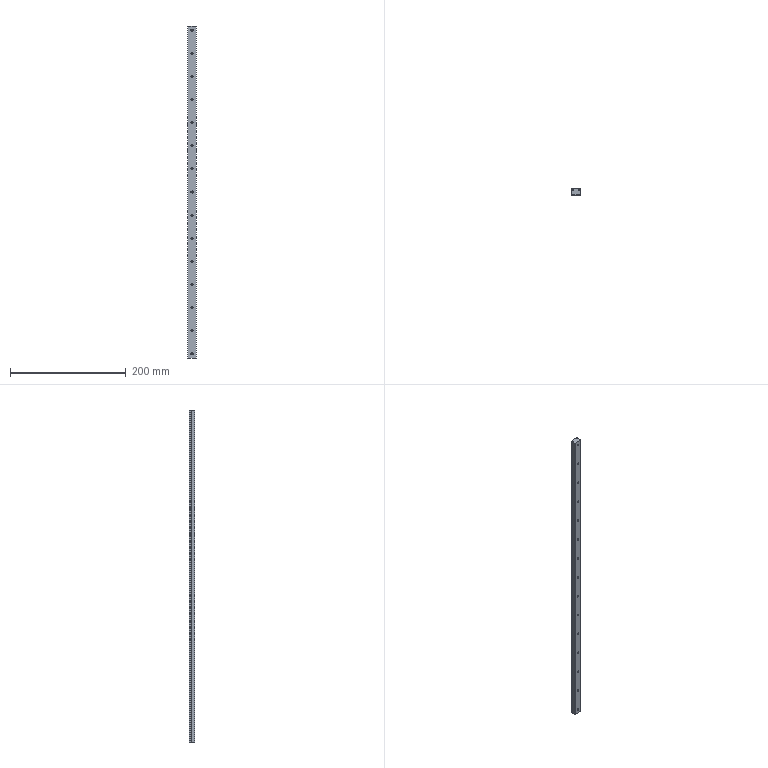Part | SolidWorks | 1 solid | 101 faces | box 15 x 10 x 574 mm | volume 77716 mm3 | cylinder 64 | plane 37 | commonest cylinder face diameters 3.5 x34 6 x30